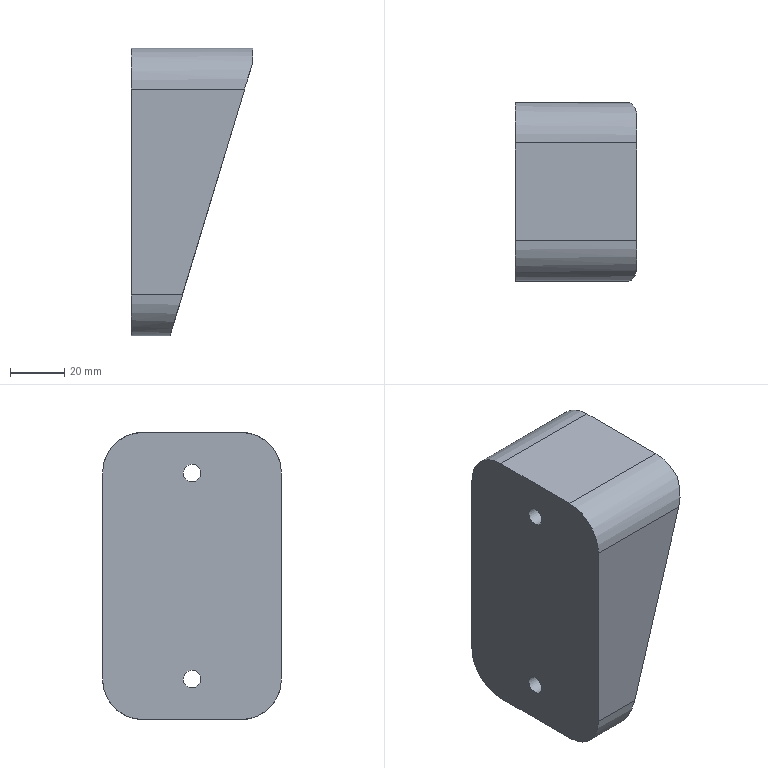Part | STEP file | solid 243 | 1 solid | 17 faces | box 45 x 66 x 106 mm | volume 203588 mm3 | plane 9 | cylinder 8 | commonest cylinder face diameters 30 x4 6.5 x2 11 x2